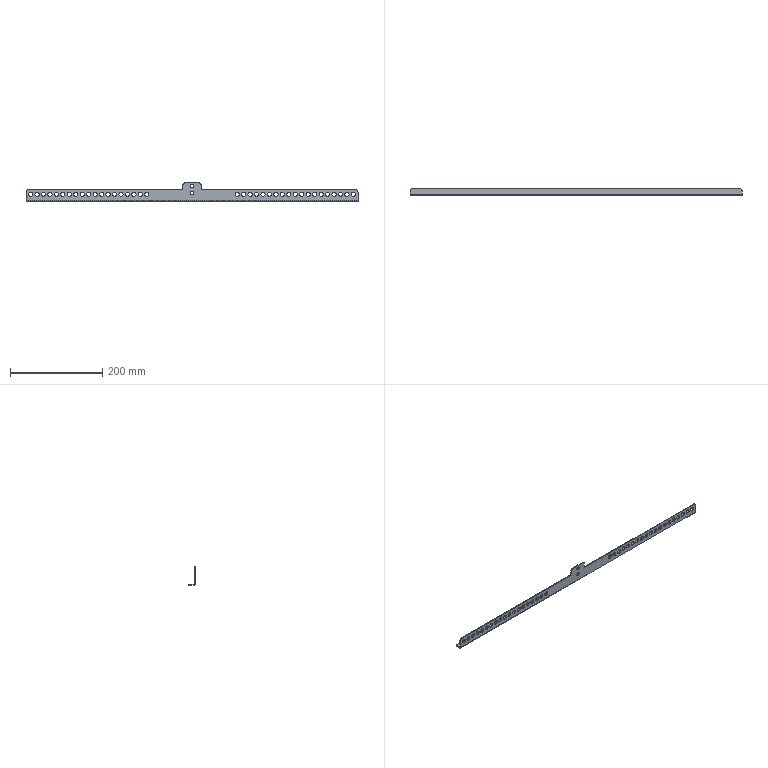Part | SolidWorks | features ICE 2, EdgeFlange 1, Fillet 1, FlatPattern 1, LPattern 1, MirrorPattern 1, SMBaseFlange 1, SheetMetal 1 | 1 solid | 104 faces | box 720 x 15 x 40 mm | volume 44933 mm3 | cylinder 88 | plane 16 | commonest cylinder face diameters 9.2 x76 10 x6 7 x4 1.473 x1 5.073 x1